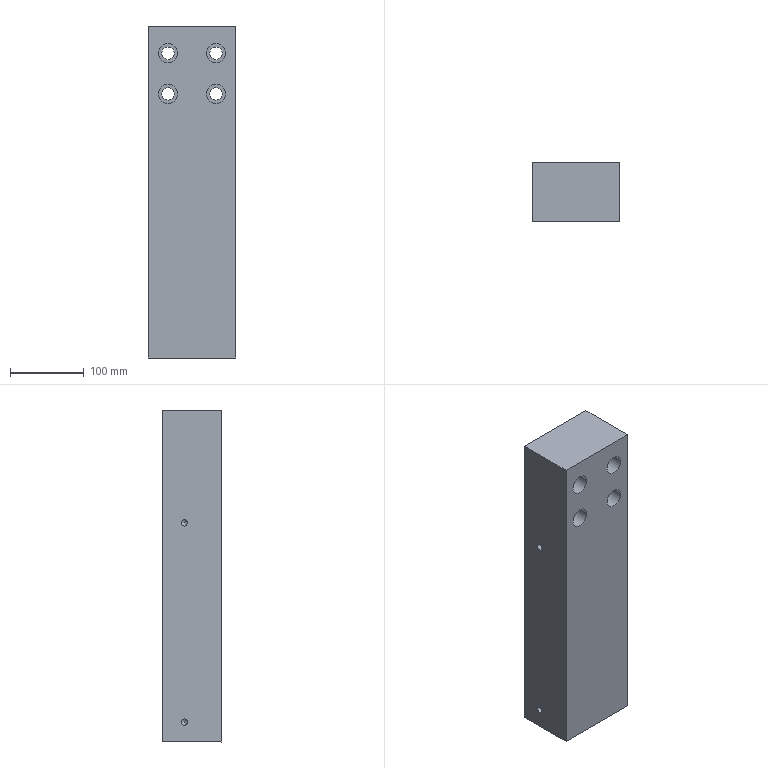Part | STEP file | lll_id1714_x_t | 1 solid | 42 faces | box 118 x 80 x 450 mm | volume 4104753 mm3 | cylinder 20 | cone 12 | plane 10 | commonest cylinder face diameters 8.5 x11 17 x4 26 x4 14 x1
STEP:
#1=CARTESIAN_POINT('',(2092.435,-628.,-262.832));
#2=VERTEX_POINT('',#1);
#3=CARTESIAN_POINT('',(2092.435,-635.,-262.832));
#4=DIRECTION('',(0.,0.000000092,-1.));
#5=DIRECTION('',(0.,1.,0.000000092));
#6=AXIS2_PLACEMENT_3D('',#3,#4,#5);
#7=CIRCLE('',#6,7.);
#8=EDGE_CURVE('',#2,#2,#7,.T.);
#9=ORIENTED_EDGE('',*,*,#8,.T.);
#10=EDGE_LOOP('',(#9));
#11=FACE_BOUND('',#10,.T.);
#12=CARTESIAN_POINT('',(2092.435,-635.,-258.626));
#13=VERTEX_POINT('',#12);
#14=VERTEX_LOOP('',#13);
#15=FACE_BOUND('',#14,.T.);
#16=CARTESIAN_POINT('',(2092.435,-635.,-262.213));
#17=DIRECTION('',(0.,0.000000092,-1.));
#18=DIRECTION('',(1.,0.,0.));
#19=AXIS2_PLACEMENT_3D('',#16,#17,#18);
#20=CONICAL_SURFACE('',#19,5.97,59.);
#21=ADVANCED_FACE('',(#11,#15),#20,.F.);
#22=CARTESIAN_POINT('',(2062.989,-625.5,9.5));
#23=VERTEX_POINT('',#22);
#24=VERTEX_LOOP('',#23);
#25=FACE_BOUND('',#24,.T.);
#26=CARTESIAN_POINT('',(2060.435,-625.5,13.75));
#27=VERTEX_POINT('',#26);
#28=CARTESIAN_POINT('',(2060.435,-625.5,9.5));
#29=DIRECTION('',(1.,0.,0.));
#30=DIRECTION('',(0.,-0.000000092,1.));
#31=AXIS2_PLACEMENT_3D('',#28,#29,#30);
#32=CIRCLE('',#31,4.25);
#33=EDGE_CURVE('',#27,#27,#32,.T.);
#34=ORIENTED_EDGE('',*,*,#33,.F.);
#35=EDGE_LOOP('',(#34));
#36=FACE_BOUND('',#35,.T.);
#37=CARTESIAN_POINT('',(2060.435,-625.5,9.5));
#38=DIRECTION('',(-1.,0.,0.));
#39=DIRECTION('',(0.,0.000000092,-1.));
#40=AXIS2_PLACEMENT_3D('',#37,#38,#39);
#41=CONICAL_SURFACE('',#40,4.25,59.);
#42=ADVANCED_FACE('',(#25,#36),#41,.F.);
#43=CARTESIAN_POINT('',(2062.989,-625.5,-260.5));
#44=VERTEX_POINT('',#43);
#45=VERTEX_LOOP('',#44);
#46=FACE_BOUND('',#45,.T.);
#47=CARTESIAN_POINT('',(2060.435,-625.5,-256.25));
#48=VERTEX_POINT('',#47);
#49=CARTESIAN_POINT('',(2060.435,-625.5,-260.5));
#50=DIRECTION('',(1.,0.,0.));
#51=DIRECTION('',(0.,-0.000000092,1.));
#52=AXIS2_PLACEMENT_3D('',#49,#50,#51);
#53=CIRCLE('',#52,4.25);
#54=EDGE_CURVE('',#48,#48,#53,.T.);
#55=ORIENTED_EDGE('',*,*,#54,.F.);
#56=EDGE_LOOP('',(#55));
#57=FACE_BOUND('',#56,.T.);
#58=CARTESIAN_POINT('',(2060.435,-625.5,-260.5));
#59=DIRECTION('',(-1.,0.,0.));
#60=DIRECTION('',(0.,0.000000092,-1.));
#61=AXIS2_PLACEMENT_3D('',#58,#59,#60);
#62=CONICAL_SURFACE('',#61,4.25,59.);
#63=ADVANCED_FACE('',(#46,#57),#62,.F.);
#64=CARTESIAN_POINT('',(2121.882,-625.5,9.5));
#65=VERTEX_POINT('',#64);
#66=VERTEX_LOOP('',#65);
#67=FACE_BOUND('',#66,.T.);
#68=CARTESIAN_POINT('',(2124.435,-625.5,13.75));
#69=VERTEX_POINT('',#68);
#70=CARTESIAN_POINT('',(2124.435,-625.5,9.5));
#71=DIRECTION('',(-1.,0.,0.));
#72=DIRECTION('',(0.,-0.000000092,1.));
#73=AXIS2_PLACEMENT_3D('',#70,#71,#72);
#74=CIRCLE('',#73,4.25);
#75=EDGE_CURVE('',#69,#69,#74,.T.);
#76=ORIENTED_EDGE('',*,*,#75,.F.);
#77=EDGE_LOOP('',(#76));
#78=FACE_BOUND('',#77,.T.);
#79=CARTESIAN_POINT('',(2124.435,-625.5,9.5));
#80=DIRECTION('',(1.,0.,0.));
#81=DIRECTION('',(0.,-0.000000092,1.));
#82=AXIS2_PLACEMENT_3D('',#79,#80,#81);
#83=CONICAL_SURFACE('',#82,4.25,59.);
#84=ADVANCED_FACE('',(#67,#78),#83,.F.);
#85=CARTESIAN_POINT('',(2121.882,-625.5,-260.5));
#86=VERTEX_POINT('',#85);
#87=VERTEX_LOOP('',#86);
#88=FACE_BOUND('',#87,.T.);
#89=CARTESIAN_POINT('',(2124.435,-625.5,-256.25));
#90=VERTEX_POINT('',#89);
#91=CARTESIAN_POINT('',(2124.435,-625.5,-260.5));
#92=DIRECTION('',(-1.,0.,0.));
#93=DIRECTION('',(0.,-0.000000092,1.));
#94=AXIS2_PLACEMENT_3D('',#91,#92,#93);
#95=CIRCLE('',#94,4.25);
#96=EDGE_CURVE('',#90,#90,#95,.T.);
#97=ORIENTED_EDGE('',*,*,#96,.F.);
#98=EDGE_LOOP('',(#97));
#99=FACE_BOUND('',#98,.T.);
#100=CARTESIAN_POINT('',(2124.435,-625.5,-260.5));
#101=DIRECTION('',(1.,0.,0.));
#102=DIRECTION('',(0.,-0.000000092,1.));
#103=AXIS2_PLACEMENT_3D('',#100,#101,#102);
#104=CONICAL_SURFACE('',#103,4.25,59.);
#105=ADVANCED_FACE('',(#88,#99),#104,.F.);
#106=CARTESIAN_POINT('',(2124.935,-636.5,83.5));
#107=VERTEX_POINT('',#106);
#108=CARTESIAN_POINT('',(2124.935,-636.5,70.5));
#109=DIRECTION('',(0.,-1.,-0.000000092));
#110=DIRECTION('',(0.,-0.000000092,1.));
#111=AXIS2_PLACEMENT_3D('',#108,#109,#110);
#112=CIRCLE('',#111,13.);
#113=EDGE_CURVE('',#107,#107,#112,.T.);
#114=ORIENTED_EDGE('',*,*,#113,.T.);
#115=EDGE_LOOP('',(#114));
#116=FACE_BOUND('',#115,.T.);
#117=CARTESIAN_POINT('',(2124.935,-636.5,79.));
#118=VERTEX_POINT('',#117);
#119=CARTESIAN_POINT('',(2124.935,-636.5,70.5));
#120=DIRECTION('',(0.,1.,0.000000092));
#121=DIRECTION('',(0.,-0.000000092,1.));
#122=AXIS2_PLACEMENT_3D('',#119,#120,#121);
#123=CIRCLE('',#122,8.5);
#124=EDGE_CURVE('',#118,#118,#123,.T.);
#125=ORIENTED_EDGE('',*,*,#124,.T.);
#126=EDGE_LOOP('',(#125));
#127=FACE_BOUND('',#126,.T.);
#128=CARTESIAN_POINT('',(2124.935,-636.5,70.5));
#129=DIRECTION('',(0.,1.,0.000000092));
#130=DIRECTION('',(0.,0.000000092,-1.));
#131=AXIS2_PLACEMENT_3D('',#128,#129,#130);
#132=PLANE('',#131);
#133=ADVANCED_FACE('',(#116,#127),#132,.F.);
#134=CARTESIAN_POINT('',(2059.935,-636.5,112.5));
#135=VERTEX_POINT('',#134);
#136=CARTESIAN_POINT('',(2059.935,-636.5,125.5));
#137=DIRECTION('',(0.,1.,0.000000092));
#138=DIRECTION('',(0.,0.000000092,-1.));
#139=AXIS2_PLACEMENT_3D('',#136,#137,#138);
#140=CIRCLE('',#139,13.);
#141=EDGE_CURVE('',#135,#135,#140,.T.);
#142=ORIENTED_EDGE('',*,*,#141,.F.);
#143=EDGE_LOOP('',(#142));
#144=FACE_BOUND('',#143,.T.);
#145=CARTESIAN_POINT('',(2059.935,-636.5,117.));
#146=VERTEX_POINT('',#145);
#147=CARTESIAN_POINT('',(2059.935,-636.5,125.5));
#148=DIRECTION('',(0.,-1.,-0.000000092));
#149=DIRECTION('',(0.,0.000000092,-1.));
#150=AXIS2_PLACEMENT_3D('',#147,#148,#149);
#151=CIRCLE('',#150,8.5);
#152=EDGE_CURVE('',#146,#146,#151,.T.);
#153=ORIENTED_EDGE('',*,*,#152,.F.);
#154=EDGE_LOOP('',(#153));
#155=FACE_BOUND('',#154,.T.);
#156=CARTESIAN_POINT('',(2059.935,-636.5,110.5));
#157=DIRECTION('',(0.,-1.,-0.000000092));
#158=DIRECTION('',(0.,-0.000000092,1.));
#159=AXIS2_PLACEMENT_3D('',#156,#157,#158);
#160=PLANE('',#159);
#161=ADVANCED_FACE('',(#144,#155),#160,.T.);
#162=CARTESIAN_POINT('',(2059.935,-636.5,57.5));
#163=VERTEX_POINT('',#162);
#164=CARTESIAN_POINT('',(2059.935,-636.5,70.5));
#165=DIRECTION('',(0.,1.,0.000000092));
#166=DIRECTION('',(0.,0.000000092,-1.));
#167=AXIS2_PLACEMENT_3D('',#164,#165,#166);
#168=CIRCLE('',#167,13.);
#169=EDGE_CURVE('',#163,#163,#168,.T.);
#170=ORIENTED_EDGE('',*,*,#169,.F.);
#171=EDGE_LOOP('',(#170));
#172=FACE_BOUND('',#171,.T.);
#173=CARTESIAN_POINT('',(2059.935,-636.5,62.));
#174=VERTEX_POINT('',#173);
#175=CARTESIAN_POINT('',(2059.935,-636.5,70.5));
#176=DIRECTION('',(0.,-1.,-0.000000092));
#177=DIRECTION('',(0.,0.000000092,-1.));
#178=AXIS2_PLACEMENT_3D('',#175,#176,#177);
#179=CIRCLE('',#178,8.5);
#180=EDGE_CURVE('',#174,#174,#179,.T.);
#181=ORIENTED_EDGE('',*,*,#180,.F.);
#182=EDGE_LOOP('',(#181));
#183=FACE_BOUND('',#182,.T.);
#184=CARTESIAN_POINT('',(2059.935,-636.5,70.5));
#185=DIRECTION('',(0.,-1.,-0.000000092));
#186=DIRECTION('',(0.,-0.000000092,1.));
#187=AXIS2_PLACEMENT_3D('',#184,#185,#186);
#188=PLANE('',#187);
#189=ADVANCED_FACE('',(#172,#183),#188,.T.);
#190=CARTESIAN_POINT('',(2124.935,-636.5,138.5));
#191=VERTEX_POINT('',#190);
#192=CARTESIAN_POINT('',(2124.935,-636.5,125.5));
#193=DIRECTION('',(0.,-1.,-0.000000092));
#194=DIRECTION('',(0.,-0.000000092,1.));
#195=AXIS2_PLACEMENT_3D('',#192,#193,#194);
#196=CIRCLE('',#195,13.);
#197=EDGE_CURVE('',#191,#191,#196,.T.);
#198=ORIENTED_EDGE('',*,*,#197,.T.);
#199=EDGE_LOOP('',(#198));
#200=FACE_BOUND('',#199,.T.);
#201=CARTESIAN_POINT('',(2124.935,-636.5,134.));
#202=VERTEX_POINT('',#201);
#203=CARTESIAN_POINT('',(2124.935,-636.5,125.5));
#204=DIRECTION('',(0.,1.,0.000000092));
#205=DIRECTION('',(0.,-0.000000092,1.));
#206=AXIS2_PLACEMENT_3D('',#203,#204,#205);
#207=CIRCLE('',#206,8.5);
#208=EDGE_CURVE('',#202,#202,#207,.T.);
#209=ORIENTED_EDGE('',*,*,#208,.T.);
#210=EDGE_LOOP('',(#209));
#211=FACE_BOUND('',#210,.T.);
#212=CARTESIAN_POINT('',(2124.935,-636.5,110.5));
#213=DIRECTION('',(0.,1.,0.000000092));
#214=DIRECTION('',(0.,0.000000092,-1.));
#215=AXIS2_PLACEMENT_3D('',#212,#213,#214);
#216=PLANE('',#215);
#217=ADVANCED_FACE('',(#200,#211),#216,.F.);
#218=ORIENTED_EDGE('',*,*,#8,.F.);
#219=EDGE_LOOP('',(#218));
#220=FACE_BOUND('',#219,.T.);
#221=CARTESIAN_POINT('',(2092.435,-642.,-287.5));
#222=VERTEX_POINT('',#221);
#223=CARTESIAN_POINT('',(2092.435,-635.,-287.5));
#224=DIRECTION('',(0.,0.000000092,-1.));
#225=DIRECTION('',(0.,-1.,-0.000000092));
#226=AXIS2_PLACEMENT_3D('',#223,#224,#225);
#227=CIRCLE('',#226,7.);
#228=EDGE_CURVE('',#222,#222,#227,.T.);
#229=ORIENTED_EDGE('',*,*,#228,.T.);
#230=EDGE_LOOP('',(#229));
#231=FACE_BOUND('',#230,.T.);
#232=CARTESIAN_POINT('',(2092.435,-635.,-255.5));
#233=DIRECTION('',(0.,-0.000000092,1.));
#234=DIRECTION('',(-1.,0.,0.));
#235=AXIS2_PLACEMENT_3D('',#232,#233,#234);
#236=CYLINDRICAL_SURFACE('',#235,7.);
#237=ADVANCED_FACE('',(#220,#231),#236,.F.);
#238=ORIENTED_EDGE('',*,*,#33,.T.);
#239=EDGE_LOOP('',(#238));
#240=FACE_BOUND('',#239,.T.);
#241=CARTESIAN_POINT('',(2033.435,-625.5,5.25));
#242=VERTEX_POINT('',#241);
#243=CARTESIAN_POINT('',(2033.435,-625.5,9.5));
#244=DIRECTION('',(1.,0.,0.));
#245=DIRECTION('',(0.,0.,-1.));
#246=AXIS2_PLACEMENT_3D('',#243,#244,#245);
#247=CIRCLE('',#246,4.25);
#248=EDGE_CURVE('',#242,#242,#247,.T.);
#249=ORIENTED_EDGE('',*,*,#248,.F.);
#250=EDGE_LOOP('',(#249));
#251=FACE_BOUND('',#250,.T.);
#252=CARTESIAN_POINT('',(2064.935,-625.5,9.5));
#253=DIRECTION('',(1.,0.,0.));
#254=DIRECTION('',(0.,-0.000000092,1.));
#255=AXIS2_PLACEMENT_3D('',#252,#253,#254);
#256=CYLINDRICAL_SURFACE('',#255,4.25);
#257=ADVANCED_FACE('',(#240,#251),#256,.F.);
#258=ORIENTED_EDGE('',*,*,#54,.T.);
#259=EDGE_LOOP('',(#258));
#260=FACE_BOUND('',#259,.T.);
#261=CARTESIAN_POINT('',(2033.435,-625.5,-264.75));
#262=VERTEX_POINT('',#261);
#263=CARTESIAN_POINT('',(2033.435,-625.5,-260.5));
#264=DIRECTION('',(1.,0.,0.));
#265=DIRECTION('',(0.,0.,-1.));
#266=AXIS2_PLACEMENT_3D('',#263,#264,#265);
#267=CIRCLE('',#266,4.25);
#268=EDGE_CURVE('',#262,#262,#267,.T.);
#269=ORIENTED_EDGE('',*,*,#268,.F.);
#270=EDGE_LOOP('',(#269));
#271=FACE_BOUND('',#270,.T.);
#272=CARTESIAN_POINT('',(2064.935,-625.5,-260.5));
#273=DIRECTION('',(1.,0.,0.));
#274=DIRECTION('',(0.,-0.000000092,1.));
#275=AXIS2_PLACEMENT_3D('',#272,#273,#274);
#276=CYLINDRICAL_SURFACE('',#275,4.25);
#277=ADVANCED_FACE('',(#260,#271),#276,.F.);
#278=ORIENTED_EDGE('',*,*,#75,.T.);
#279=EDGE_LOOP('',(#278));
#280=FACE_BOUND('',#279,.T.);
#281=CARTESIAN_POINT('',(2151.435,-625.5,13.75));
#282=VERTEX_POINT('',#281);
#283=CARTESIAN_POINT('',(2151.435,-625.5,9.5));
#284=DIRECTION('',(-1.,0.,0.));
#285=DIRECTION('',(0.,0.,1.));
#286=AXIS2_PLACEMENT_3D('',#283,#284,#285);
#287=CIRCLE('',#286,4.25);
#288=EDGE_CURVE('',#282,#282,#287,.T.);
#289=ORIENTED_EDGE('',*,*,#288,.F.);
#290=EDGE_LOOP('',(#289));
#291=FACE_BOUND('',#290,.T.);
#292=CARTESIAN_POINT('',(2119.935,-625.5,9.5));
#293=DIRECTION('',(-1.,0.,0.));
#294=DIRECTION('',(0.,0.000000092,-1.));
#295=AXIS2_PLACEMENT_3D('',#292,#293,#294);
#296=CYLINDRICAL_SURFACE('',#295,4.25);
#297=ADVANCED_FACE('',(#280,#291),#296,.F.);
#298=ORIENTED_EDGE('',*,*,#96,.T.);
#299=EDGE_LOOP('',(#298));
#300=FACE_BOUND('',#299,.T.);
#301=CARTESIAN_POINT('',(2151.435,-625.5,-256.25));
#302=VERTEX_POINT('',#301);
#303=CARTESIAN_POINT('',(2151.435,-625.5,-260.5));
#304=DIRECTION('',(-1.,0.,0.));
#305=DIRECTION('',(0.,0.,1.));
#306=AXIS2_PLACEMENT_3D('',#303,#304,#305);
#307=CIRCLE('',#306,4.25);
#308=EDGE_CURVE('',#302,#302,#307,.T.);
#309=ORIENTED_EDGE('',*,*,#308,.F.);
#310=EDGE_LOOP('',(#309));
#311=FACE_BOUND('',#310,.T.);
#312=CARTESIAN_POINT('',(2119.935,-625.5,-260.5));
#313=DIRECTION('',(-1.,0.,0.));
#314=DIRECTION('',(0.,0.000000092,-1.));
#315=AXIS2_PLACEMENT_3D('',#312,#313,#314);
#316=CYLINDRICAL_SURFACE('',#315,4.25);
#317=ADVANCED_FACE('',(#300,#311),#316,.F.);
#318=ORIENTED_EDGE('',*,*,#124,.F.);
#319=EDGE_LOOP('',(#318));
#320=FACE_BOUND('',#319,.T.);
#321=CARTESIAN_POINT('',(2124.935,-596.,62.));
#322=VERTEX_POINT('',#321);
#323=CARTESIAN_POINT('',(2124.935,-596.,70.5));
#324=DIRECTION('',(0.,1.,0.000000092));
#325=DIRECTION('',(0.,0.000000092,-1.));
#326=AXIS2_PLACEMENT_3D('',#323,#324,#325);
#327=CIRCLE('',#326,8.5);
#328=EDGE_CURVE('',#322,#322,#327,.T.);
#329=ORIENTED_EDGE('',*,*,#328,.T.);
#330=EDGE_LOOP('',(#329));
#331=FACE_BOUND('',#330,.T.);
#332=CARTESIAN_POINT('',(2124.935,-649.5,70.5));
#333=DIRECTION('',(0.,1.,0.000000092));
#334=DIRECTION('',(0.,0.000000092,-1.));
#335=AXIS2_PLACEMENT_3D('',#332,#333,#334);
#336=CYLINDRICAL_SURFACE('',#335,8.5);
#337=ADVANCED_FACE('',(#320,#331),#336,.F.);
#338=ORIENTED_EDGE('',*,*,#152,.T.);
#339=EDGE_LOOP('',(#338));
#340=FACE_BOUND('',#339,.T.);
#341=CARTESIAN_POINT('',(2059.935,-596.,117.));
#342=VERTEX_POINT('',#341);
#343=CARTESIAN_POINT('',(2059.935,-596.,125.5));
#344=DIRECTION('',(0.,1.,0.000000092));
#345=DIRECTION('',(0.,0.000000092,-1.));
#346=AXIS2_PLACEMENT_3D('',#343,#344,#345);
#347=CIRCLE('',#346,8.5);
#348=EDGE_CURVE('',#342,#342,#347,.T.);
#349=ORIENTED_EDGE('',*,*,#348,.T.);
#350=EDGE_LOOP('',(#349));
#351=FACE_BOUND('',#350,.T.);
#352=CARTESIAN_POINT('',(2059.935,-649.5,125.5));
#353=DIRECTION('',(0.,1.,0.000000092));
#354=DIRECTION('',(0.,0.000000092,-1.));
#355=AXIS2_PLACEMENT_3D('',#352,#353,#354);
#356=CYLINDRICAL_SURFACE('',#355,8.5);
#357=ADVANCED_FACE('',(#340,#351),#356,.F.);
#358=ORIENTED_EDGE('',*,*,#180,.T.);
#359=EDGE_LOOP('',(#358));
#360=FACE_BOUND('',#359,.T.);
#361=CARTESIAN_POINT('',(2059.935,-596.,62.));
#362=VERTEX_POINT('',#361);
#363=CARTESIAN_POINT('',(2059.935,-596.,70.5));
#364=DIRECTION('',(0.,1.,0.000000092));
#365=DIRECTION('',(0.,0.000000092,-1.));
#366=AXIS2_PLACEMENT_3D('',#363,#364,#365);
#367=CIRCLE('',#366,8.5);
#368=EDGE_CURVE('',#362,#362,#367,.T.);
#369=ORIENTED_EDGE('',*,*,#368,.T.);
#370=EDGE_LOOP('',(#369));
#371=FACE_BOUND('',#370,.T.);
#372=CARTESIAN_POINT('',(2059.935,-649.5,70.5));
#373=DIRECTION('',(0.,1.,0.000000092));
#374=DIRECTION('',(0.,0.000000092,-1.));
#375=AXIS2_PLACEMENT_3D('',#372,#373,#374);
#376=CYLINDRICAL_SURFACE('',#375,8.5);
#377=ADVANCED_FACE('',(#360,#371),#376,.F.);
#378=ORIENTED_EDGE('',*,*,#208,.F.);
#379=EDGE_LOOP('',(#378));
#380=FACE_BOUND('',#379,.T.);
#381=CARTESIAN_POINT('',(2124.935,-596.,117.));
#382=VERTEX_POINT('',#381);
#383=CARTESIAN_POINT('',(2124.935,-596.,125.5));
#384=DIRECTION('',(0.,1.,0.000000092));
#385=DIRECTION('',(0.,0.000000092,-1.));
#386=AXIS2_PLACEMENT_3D('',#383,#384,#385);
#387=CIRCLE('',#386,8.5);
#388=EDGE_CURVE('',#382,#382,#387,.T.);
#389=ORIENTED_EDGE('',*,*,#388,.T.);
#390=EDGE_LOOP('',(#389));
#391=FACE_BOUND('',#390,.T.);
#392=CARTESIAN_POINT('',(2124.935,-649.5,125.5));
#393=DIRECTION('',(0.,1.,0.000000092));
#394=DIRECTION('',(0.,0.000000092,-1.));
#395=AXIS2_PLACEMENT_3D('',#392,#393,#394);
#396=CYLINDRICAL_SURFACE('',#395,8.5);
#397=ADVANCED_FACE('',(#380,#391),#396,.F.);
#398=ORIENTED_EDGE('',*,*,#228,.F.);
#399=EDGE_LOOP('',(#398));
#400=FACE_BOUND('',#399,.T.);
#401=CARTESIAN_POINT('',(2151.435,-676.,-287.5));
#402=VERTEX_POINT('',#401);
#403=CARTESIAN_POINT('',(2151.435,-596.,-287.5));
#404=VERTEX_POINT('',#403);
#405=CARTESIAN_POINT('',(2151.435,-604.571,-287.5));
#406=DIRECTION('',(0.,1.,0.000000092));
#407=VECTOR('',#406,1.);
#408=LINE('',#405,#407);
#409=EDGE_CURVE('',#402,#404,#408,.T.);
#410=ORIENTED_EDGE('',*,*,#409,.F.);
#411=CARTESIAN_POINT('',(2033.435,-676.,-287.5));
#412=VERTEX_POINT('',#411);
#413=CARTESIAN_POINT('',(2029.935,-676.,-287.5));
#414=DIRECTION('',(-1.,0.,0.));
#415=VECTOR('',#414,1.);
#416=LINE('',#413,#415);
#417=EDGE_CURVE('',#402,#412,#416,.T.);
#418=ORIENTED_EDGE('',*,*,#417,.T.);
#419=CARTESIAN_POINT('',(2033.435,-596.,-287.5));
#420=VERTEX_POINT('',#419);
#421=CARTESIAN_POINT('',(2033.435,-604.571,-287.5));
#422=DIRECTION('',(0.,-1.,-0.000000092));
#423=VECTOR('',#422,1.);
#424=LINE('',#421,#423);
#425=EDGE_CURVE('',#420,#412,#424,.T.);
#426=ORIENTED_EDGE('',*,*,#425,.F.);
#427=CARTESIAN_POINT('',(2149.935,-596.,-287.5));
#428=DIRECTION('',(1.,0.,0.));
#429=VECTOR('',#428,1.);
#430=LINE('',#427,#429);
#431=EDGE_CURVE('',#420,#404,#430,.T.);
#432=ORIENTED_EDGE('',*,*,#431,.T.);
#433=EDGE_LOOP('',(#410,#418,#426,#432));
#434=FACE_BOUND('',#433,.T.);
#435=CARTESIAN_POINT('',(2149.935,-604.571,-287.5));
#436=DIRECTION('',(0.,-0.000000092,1.));
#437=DIRECTION('',(-1.,0.,0.));
#438=AXIS2_PLACEMENT_3D('',#435,#436,#437);
#439=PLANE('',#438);
#440=ADVANCED_FACE('',(#400,#434),#439,.F.);
#441=ORIENTED_EDGE('',*,*,#268,.T.);
#442=EDGE_LOOP('',(#441));
#443=FACE_BOUND('',#442,.T.);
#444=ORIENTED_EDGE('',*,*,#248,.T.);
#445=EDGE_LOOP('',(#444));
#446=FACE_BOUND('',#445,.T.);
#447=CARTESIAN_POINT('',(2033.435,-596.,162.5));
#448=VERTEX_POINT('',#447);
#449=CARTESIAN_POINT('',(2033.435,-596.,-85.484));
#450=DIRECTION('',(0.,0.000000092,-1.));
#451=VECTOR('',#450,1.);
#452=LINE('',#449,#451);
#453=EDGE_CURVE('',#448,#420,#452,.T.);
#454=ORIENTED_EDGE('',*,*,#453,.T.);
#455=ORIENTED_EDGE('',*,*,#425,.T.);
#456=CARTESIAN_POINT('',(2033.435,-676.,162.5));
#457=VERTEX_POINT('',#456);
#458=CARTESIAN_POINT('',(2033.435,-676.,180.5));
#459=DIRECTION('',(0.,0.000000092,-1.));
#460=VECTOR('',#459,1.);
#461=LINE('',#458,#460);
#462=EDGE_CURVE('',#457,#412,#461,.T.);
#463=ORIENTED_EDGE('',*,*,#462,.F.);
#464=CARTESIAN_POINT('',(2033.435,-549.5,162.5));
#465=DIRECTION('',(0.,-1.,-0.000000092));
#466=VECTOR('',#465,1.);
#467=LINE('',#464,#466);
#468=EDGE_CURVE('',#448,#457,#467,.T.);
#469=ORIENTED_EDGE('',*,*,#468,.F.);
#470=EDGE_LOOP('',(#454,#455,#463,#469));
#471=FACE_BOUND('',#470,.T.);
#472=CARTESIAN_POINT('',(2033.435,-549.5,-85.484));
#473=DIRECTION('',(-1.,0.,0.));
#474=DIRECTION('',(0.,0.000000092,-1.));
#475=AXIS2_PLACEMENT_3D('',#472,#473,#474);
#476=PLANE('',#475);
#477=ADVANCED_FACE('',(#443,#446,#471),#476,.T.);
#478=ORIENTED_EDGE('',*,*,#468,.T.);
#479=CARTESIAN_POINT('',(2151.435,-676.,162.5));
#480=VERTEX_POINT('',#479);
#481=CARTESIAN_POINT('',(2029.935,-676.,162.5));
#482=DIRECTION('',(-1.,0.,0.));
#483=VECTOR('',#482,1.);
#484=LINE('',#481,#483);
#485=EDGE_CURVE('',#480,#457,#484,.T.);
#486=ORIENTED_EDGE('',*,*,#485,.F.);
#487=CARTESIAN_POINT('',(2151.435,-596.,162.5));
#488=VERTEX_POINT('',#487);
#489=CARTESIAN_POINT('',(2151.435,-574.,162.5));
#490=DIRECTION('',(0.,-1.,-0.000000092));
#491=VECTOR('',#490,1.);
#492=LINE('',#489,#491);
#493=EDGE_CURVE('',#488,#480,#492,.T.);
#494=ORIENTED_EDGE('',*,*,#493,.F.);
#495=CARTESIAN_POINT('',(2157.935,-596.,162.5));
#496=DIRECTION('',(1.,0.,0.));
#497=VECTOR('',#496,1.);
#498=LINE('',#495,#497);
#499=EDGE_CURVE('',#448,#488,#498,.T.);
#500=ORIENTED_EDGE('',*,*,#499,.F.);
#501=EDGE_LOOP('',(#478,#486,#494,#500));
#502=FACE_OUTER_BOUND('',#501,.T.);
#503=CARTESIAN_POINT('',(2034.935,-574.,162.5));
#504=DIRECTION('',(0.,-0.000000092,1.));
#505=DIRECTION('',(1.,0.,0.));
#506=AXIS2_PLACEMENT_3D('',#503,#504,#505);
#507=PLANE('',#506);
#508=ADVANCED_FACE('',(#502),#507,.T.);
#509=CARTESIAN_POINT('',(2151.435,-625.5,-121.25));
#510=VERTEX_POINT('',#509);
#511=CARTESIAN_POINT('',(2151.435,-625.5,-125.5));
#512=DIRECTION('',(-1.,0.,0.));
#513=DIRECTION('',(0.,0.,1.));
#514=AXIS2_PLACEMENT_3D('',#511,#512,#513);
#515=CIRCLE('',#514,4.25);
#516=EDGE_CURVE('',#510,#510,#515,.T.);
#517=ORIENTED_EDGE('',*,*,#516,.T.);
#518=EDGE_LOOP('',(#517));
#519=FACE_BOUND('',#518,.T.);
#520=ORIENTED_EDGE('',*,*,#308,.T.);
#521=EDGE_LOOP('',(#520));
#522=FACE_BOUND('',#521,.T.);
#523=ORIENTED_EDGE('',*,*,#288,.T.);
#524=EDGE_LOOP('',(#523));
#525=FACE_BOUND('',#524,.T.);
#526=CARTESIAN_POINT('',(2151.435,-676.,180.5));
#527=DIRECTION('',(0.,-0.000000092,1.));
#528=VECTOR('',#527,1.);
#529=LINE('',#526,#528);
#530=EDGE_CURVE('',#402,#480,#529,.T.);
#531=ORIENTED_EDGE('',*,*,#530,.F.);
#532=ORIENTED_EDGE('',*,*,#409,.T.);
#533=CARTESIAN_POINT('',(2151.435,-596.,24.5));
#534=DIRECTION('',(0.,0.000000092,-1.));
#535=VECTOR('',#534,1.);
#536=LINE('',#533,#535);
#537=EDGE_CURVE('',#488,#404,#536,.T.);
#538=ORIENTED_EDGE('',*,*,#537,.F.);
#539=ORIENTED_EDGE('',*,*,#493,.T.);
#540=EDGE_LOOP('',(#531,#532,#538,#539));
#541=FACE_BOUND('',#540,.T.);
#542=CARTESIAN_POINT('',(2151.435,-549.5,49.509));
#543=DIRECTION('',(1.,0.,0.));
#544=DIRECTION('',(0.,-0.000000092,1.));
#545=AXIS2_PLACEMENT_3D('',#542,#543,#544);
#546=PLANE('',#545);
#547=ADVANCED_FACE('',(#519,#522,#525,#541),#546,.T.);
#548=CARTESIAN_POINT('',(2067.435,-596.,-103.75));
#549=VERTEX_POINT('',#548);
#550=CARTESIAN_POINT('',(2067.435,-596.,-108.));
#551=DIRECTION('',(0.,1.,0.000000092));
#552=DIRECTION('',(0.,-0.000000092,1.));
#553=AXIS2_PLACEMENT_3D('',#550,#551,#552);
#554=CIRCLE('',#553,4.25);
#555=EDGE_CURVE('',#549,#549,#554,.T.);
#556=ORIENTED_EDGE('',*,*,#555,.F.);
#557=EDGE_LOOP('',(#556));
#558=FACE_BOUND('',#557,.T.);
#559=CARTESIAN_POINT('',(2117.435,-596.,-103.75));
#560=VERTEX_POINT('',#559);
#561=CARTESIAN_POINT('',(2117.435,-596.,-108.));
#562=DIRECTION('',(0.,1.,0.000000092));
#563=DIRECTION('',(0.,-0.000000092,1.));
#564=AXIS2_PLACEMENT_3D('',#561,#562,#563);
#565=CIRCLE('',#564,4.25);
#566=EDGE_CURVE('',#560,#560,#565,.T.);
#567=ORIENTED_EDGE('',*,*,#566,.F.);
#568=EDGE_LOOP('',(#567));
#569=FACE_BOUND('',#568,.T.);
#570=CARTESIAN_POINT('',(2067.435,-596.,23.75));
#571=VERTEX_POINT('',#570);
#572=CARTESIAN_POINT('',(2067.435,-596.,19.5));
#573=DIRECTION('',(0.,1.,0.000000092));
#574=DIRECTION('',(0.,-0.000000092,1.));
#575=AXIS2_PLACEMENT_3D('',#572,#573,#574);
#576=CIRCLE('',#575,4.25);
#577=EDGE_CURVE('',#571,#571,#576,.T.);
#578=ORIENTED_EDGE('',*,*,#577,.F.);
#579=EDGE_LOOP('',(#578));
#580=FACE_BOUND('',#579,.T.);
#581=CARTESIAN_POINT('',(2117.435,-596.,23.75));
#582=VERTEX_POINT('',#581);
#583=CARTESIAN_POINT('',(2117.435,-596.,19.5));
#584=DIRECTION('',(0.,1.,0.000000092));
#585=DIRECTION('',(0.,-0.000000092,1.));
#586=AXIS2_PLACEMENT_3D('',#583,#584,#585);
#587=CIRCLE('',#586,4.25);
#588=EDGE_CURVE('',#582,#582,#587,.T.);
#589=ORIENTED_EDGE('',*,*,#588,.F.);
#590=EDGE_LOOP('',(#589));
#591=FACE_BOUND('',#590,.T.);
#592=CARTESIAN_POINT('',(2117.435,-596.,-241.25));
#593=VERTEX_POINT('',#592);
#594=CARTESIAN_POINT('',(2117.435,-596.,-245.5));
#595=DIRECTION('',(0.,1.,0.000000092));
#596=DIRECTION('',(0.,-0.000000092,1.));
#597=AXIS2_PLACEMENT_3D('',#594,#595,#596);
#598=CIRCLE('',#597,4.25);
#599=EDGE_CURVE('',#593,#593,#598,.T.);
#600=ORIENTED_EDGE('',*,*,#599,.F.);
#601=EDGE_LOOP('',(#600));
#602=FACE_BOUND('',#601,.T.);
#603=CARTESIAN_POINT('',(2067.435,-596.,-241.25));
#604=VERTEX_POINT('',#603);
#605=CARTESIAN_POINT('',(2067.435,-596.,-245.5));
#606=DIRECTION('',(0.,1.,0.000000092));
#607=DIRECTION('',(0.,-0.000000092,1.));
#608=AXIS2_PLACEMENT_3D('',#605,#606,#607);
#609=CIRCLE('',#608,4.25);
#610=EDGE_CURVE('',#604,#604,#609,.T.);
#611=ORIENTED_EDGE('',*,*,#610,.F.);
#612=EDGE_LOOP('',(#611));
#613=FACE_BOUND('',#612,.T.);
#614=ORIENTED_EDGE('',*,*,#537,.T.);
#615=ORIENTED_EDGE('',*,*,#431,.F.);
#616=ORIENTED_EDGE('',*,*,#453,.F.);
#617=ORIENTED_EDGE('',*,*,#499,.T.);
#618=EDGE_LOOP('',(#614,#615,#616,#617));
#619=FACE_BOUND('',#618,.T.);
#620=ORIENTED_EDGE('',*,*,#388,.F.);
#621=EDGE_LOOP('',(#620));
#622=FACE_BOUND('',#621,.T.);
#623=ORIENTED_EDGE('',*,*,#368,.F.);
#624=EDGE_LOOP('',(#623));
#625=FACE_BOUND('',#624,.T.);
#626=ORIENTED_EDGE('',*,*,#348,.F.);
#627=EDGE_LOOP('',(#626));
#628=FACE_BOUND('',#627,.T.);
#629=ORIENTED_EDGE('',*,*,#328,.F.);
#630=EDGE_LOOP('',(#629));
#631=FACE_BOUND('',#630,.T.);
#632=CARTESIAN_POINT('',(2157.935,-596.,24.5));
#633=DIRECTION('',(0.,-1.,-0.000000092));
#634=DIRECTION('',(0.,0.000000092,-1.));
#635=AXIS2_PLACEMENT_3D('',#632,#633,#634);
#636=PLANE('',#635);
#637=ADVANCED_FACE('',(#558,#569,#580,#591,#602,#613,#619,#622,#625,#628,#631),#636,.F.);
#638=CARTESIAN_POINT('',(2059.935,-676.,57.5));
#639=VERTEX_POINT('',#638);
#640=CARTESIAN_POINT('',(2059.935,-676.,70.5));
#641=DIRECTION('',(0.,-1.,-0.000000092));
#642=DIRECTION('',(0.,0.000000092,-1.));
#643=AXIS2_PLACEMENT_3D('',#640,#641,#642);
#644=CIRCLE('',#643,13.);
#645=EDGE_CURVE('',#639,#639,#644,.T.);
#646=ORIENTED_EDGE('',*,*,#645,.T.);
#647=EDGE_LOOP('',(#646));
#648=FACE_BOUND('',#647,.T.);
#649=ORIENTED_EDGE('',*,*,#169,.T.);
#650=EDGE_LOOP('',(#649));
#651=FACE_BOUND('',#650,.T.);
#652=CARTESIAN_POINT('',(2059.935,-649.5,70.5));
#653=DIRECTION('',(0.,1.,0.000000092));
#654=DIRECTION('',(0.,0.000000092,-1.));
#655=AXIS2_PLACEMENT_3D('',#652,#653,#654);
#656=CYLINDRICAL_SURFACE('',#655,13.);
#657=ADVANCED_FACE('',(#648,#651),#656,.F.);
#658=CARTESIAN_POINT('',(2124.935,-676.,57.5));
#659=VERTEX_POINT('',#658);
#660=CARTESIAN_POINT('',(2124.935,-676.,70.5));
#661=DIRECTION('',(0.,1.,0.000000092));
#662=DIRECTION('',(0.,0.000000092,-1.));
#663=AXIS2_PLACEMENT_3D('',#660,#661,#662);
#664=CIRCLE('',#663,13.);
#665=EDGE_CURVE('',#659,#659,#664,.T.);
#666=ORIENTED_EDGE('',*,*,#665,.F.);
#667=EDGE_LOOP('',(#666));
#668=FACE_BOUND('',#667,.T.);
#669=ORIENTED_EDGE('',*,*,#113,.F.);
#670=EDGE_LOOP('',(#669));
#671=FACE_BOUND('',#670,.T.);
#672=CARTESIAN_POINT('',(2124.935,-649.5,70.5));
#673=DIRECTION('',(0.,1.,0.000000092));
#674=DIRECTION('',(0.,0.000000092,-1.));
#675=AXIS2_PLACEMENT_3D('',#672,#673,#674);
#676=CYLINDRICAL_SURFACE('',#675,13.);
#677=ADVANCED_FACE('',(#668,#671),#676,.F.);
#678=CARTESIAN_POINT('',(2059.935,-676.,112.5));
#679=VERTEX_POINT('',#678);
#680=CARTESIAN_POINT('',(2059.935,-676.,125.5));
#681=DIRECTION('',(0.,1.,0.000000092));
#682=DIRECTION('',(0.,0.000000092,-1.));
#683=AXIS2_PLACEMENT_3D('',#680,#681,#682);
#684=CIRCLE('',#683,13.);
#685=EDGE_CURVE('',#679,#679,#684,.T.);
#686=ORIENTED_EDGE('',*,*,#685,.F.);
#687=EDGE_LOOP('',(#686));
#688=FACE_BOUND('',#687,.T.);
#689=ORIENTED_EDGE('',*,*,#141,.T.);
#690=EDGE_LOOP('',(#689));
#691=FACE_BOUND('',#690,.T.);
#692=CARTESIAN_POINT('',(2059.935,-649.5,125.5));
#693=DIRECTION('',(0.,1.,0.000000092));
#694=DIRECTION('',(0.,0.000000092,-1.));
#695=AXIS2_PLACEMENT_3D('',#692,#693,#694);
#696=CYLINDRICAL_SURFACE('',#695,13.);
#697=ADVANCED_FACE('',(#688,#691),#696,.F.);
#698=CARTESIAN_POINT('',(2124.935,-676.,112.5));
#699=VERTEX_POINT('',#698);
#700=CARTESIAN_POINT('',(2124.935,-676.,125.5));
#701=DIRECTION('',(0.,-1.,-0.000000092));
#702=DIRECTION('',(0.,0.000000092,-1.));
#703=AXIS2_PLACEMENT_3D('',#700,#701,#702);
#704=CIRCLE('',#703,13.);
#705=EDGE_CURVE('',#699,#699,#704,.T.);
#706=ORIENTED_EDGE('',*,*,#705,.T.);
#707=EDGE_LOOP('',(#706));
#708=FACE_BOUND('',#707,.T.);
#709=ORIENTED_EDGE('',*,*,#197,.F.);
#710=EDGE_LOOP('',(#709));
#711=FACE_BOUND('',#710,.T.);
#712=CARTESIAN_POINT('',(2124.935,-649.5,125.5));
#713=DIRECTION('',(0.,1.,0.000000092));
#714=DIRECTION('',(0.,0.000000092,-1.));
#715=AXIS2_PLACEMENT_3D('',#712,#713,#714);
#716=CYLINDRICAL_SURFACE('',#715,13.);
#717=ADVANCED_FACE('',(#708,#711),#716,.F.);
#718=ORIENTED_EDGE('',*,*,#705,.F.);
#719=EDGE_LOOP('',(#718));
#720=FACE_BOUND('',#719,.T.);
#721=ORIENTED_EDGE('',*,*,#685,.T.);
#722=EDGE_LOOP('',(#721));
#723=FACE_BOUND('',#722,.T.);
#724=ORIENTED_EDGE('',*,*,#665,.T.);
#725=EDGE_LOOP('',(#724));
#726=FACE_BOUND('',#725,.T.);
#727=ORIENTED_EDGE('',*,*,#645,.F.);
#728=EDGE_LOOP('',(#727));
#729=FACE_BOUND('',#728,.T.);
#730=ORIENTED_EDGE('',*,*,#462,.T.);
#731=ORIENTED_EDGE('',*,*,#417,.F.);
#732=ORIENTED_EDGE('',*,*,#530,.T.);
#733=ORIENTED_EDGE('',*,*,#485,.T.);
#734=EDGE_LOOP('',(#730,#731,#732,#733));
#735=FACE_BOUND('',#734,.T.);
#736=CARTESIAN_POINT('',(2029.935,-676.,180.5));
#737=DIRECTION('',(0.,1.,0.000000092));
#738=DIRECTION('',(0.,0.000000092,-1.));
#739=AXIS2_PLACEMENT_3D('',#736,#737,#738);
#740=PLANE('',#739);
#741=ADVANCED_FACE('',(#720,#723,#726,#729,#735),#740,.F.);
#742=CARTESIAN_POINT('',(2121.435,-625.5,-121.25));
#743=VERTEX_POINT('',#742);
#744=CARTESIAN_POINT('',(2121.435,-625.5,-125.5));
#745=DIRECTION('',(1.,0.,0.));
#746=DIRECTION('',(0.,0.,1.));
#747=AXIS2_PLACEMENT_3D('',#744,#745,#746);
#748=CIRCLE('',#747,4.25);
#749=EDGE_CURVE('',#743,#743,#748,.T.);
#750=ORIENTED_EDGE('',*,*,#749,.T.);
#751=EDGE_LOOP('',(#750));
#752=FACE_BOUND('',#751,.T.);
#753=CARTESIAN_POINT('',(2118.882,-625.5,-125.5));
#754=VERTEX_POINT('',#753);
#755=VERTEX_LOOP('',#754);
#756=FACE_BOUND('',#755,.T.);
#757=CARTESIAN_POINT('',(2121.435,-625.5,-125.5));
#758=DIRECTION('',(1.,0.,0.));
#759=DIRECTION('',(0.,0.,-1.));
#760=AXIS2_PLACEMENT_3D('',#757,#758,#759);
#761=CONICAL_SURFACE('',#760,4.25,59.);
#762=ADVANCED_FACE('',(#752,#756),#761,.F.);
#763=ORIENTED_EDGE('',*,*,#749,.F.);
#764=EDGE_LOOP('',(#763));
#765=FACE_BOUND('',#764,.T.);
#766=ORIENTED_EDGE('',*,*,#516,.F.);
#767=EDGE_LOOP('',(#766));
#768=FACE_BOUND('',#767,.T.);
#769=CARTESIAN_POINT('',(2151.435,-625.5,-125.5));
#770=DIRECTION('',(-1.,0.,0.));
#771=DIRECTION('',(0.,0.,1.));
#772=AXIS2_PLACEMENT_3D('',#769,#770,#771);
#773=CYLINDRICAL_SURFACE('',#772,4.25);
#774=ADVANCED_FACE('',(#765,#768),#773,.F.);
#775=CARTESIAN_POINT('',(2067.435,-626.,-241.25));
#776=VERTEX_POINT('',#775);
#777=CARTESIAN_POINT('',(2067.435,-626.,-245.5));
#778=DIRECTION('',(0.,-1.,-0.000000092));
#779=DIRECTION('',(0.,-0.000000092,1.));
#780=AXIS2_PLACEMENT_3D('',#777,#778,#779);
#781=CIRCLE('',#780,4.25);
#782=EDGE_CURVE('',#776,#776,#781,.T.);
#783=ORIENTED_EDGE('',*,*,#782,.F.);
#784=EDGE_LOOP('',(#783));
#785=FACE_BOUND('',#784,.T.);
#786=CARTESIAN_POINT('',(2067.435,-628.554,-245.5));
#787=VERTEX_POINT('',#786);
#788=VERTEX_LOOP('',#787);
#789=FACE_BOUND('',#788,.T.);
#790=CARTESIAN_POINT('',(2067.435,-626.,-245.5));
#791=DIRECTION('',(0.,1.,0.000000092));
#792=DIRECTION('',(0.,0.000000092,-1.));
#793=AXIS2_PLACEMENT_3D('',#790,#791,#792);
#794=CONICAL_SURFACE('',#793,4.25,59.);
#795=ADVANCED_FACE('',(#785,#789),#794,.F.);
#796=ORIENTED_EDGE('',*,*,#782,.T.);
#797=EDGE_LOOP('',(#796));
#798=FACE_BOUND('',#797,.T.);
#799=ORIENTED_EDGE('',*,*,#610,.T.);
#800=EDGE_LOOP('',(#799));
#801=FACE_BOUND('',#800,.T.);
#802=CARTESIAN_POINT('',(2067.435,-596.,-245.5));
#803=DIRECTION('',(0.,-1.,-0.000000092));
#804=DIRECTION('',(0.,-0.000000092,1.));
#805=AXIS2_PLACEMENT_3D('',#802,#803,#804);
#806=CYLINDRICAL_SURFACE('',#805,4.25);
#807=ADVANCED_FACE('',(#798,#801),#806,.F.);
#808=CARTESIAN_POINT('',(2117.435,-626.,-241.25));
#809=VERTEX_POINT('',#808);
#810=CARTESIAN_POINT('',(2117.435,-626.,-245.5));
#811=DIRECTION('',(0.,-1.,-0.000000092));
#812=DIRECTION('',(0.,-0.000000092,1.));
#813=AXIS2_PLACEMENT_3D('',#810,#811,#812);
#814=CIRCLE('',#813,4.25);
#815=EDGE_CURVE('',#809,#809,#814,.T.);
#816=ORIENTED_EDGE('',*,*,#815,.F.);
#817=EDGE_LOOP('',(#816));
#818=FACE_BOUND('',#817,.T.);
#819=CARTESIAN_POINT('',(2117.435,-628.554,-245.5));
#820=VERTEX_POINT('',#819);
#821=VERTEX_LOOP('',#820);
#822=FACE_BOUND('',#821,.T.);
#823=CARTESIAN_POINT('',(2117.435,-626.,-245.5));
#824=DIRECTION('',(0.,1.,0.000000092));
#825=DIRECTION('',(0.,0.000000092,-1.));
#826=AXIS2_PLACEMENT_3D('',#823,#824,#825);
#827=CONICAL_SURFACE('',#826,4.25,59.);
#828=ADVANCED_FACE('',(#818,#822),#827,.F.);
#829=ORIENTED_EDGE('',*,*,#815,.T.);
#830=EDGE_LOOP('',(#829));
#831=FACE_BOUND('',#830,.T.);
#832=ORIENTED_EDGE('',*,*,#599,.T.);
#833=EDGE_LOOP('',(#832));
#834=FACE_BOUND('',#833,.T.);
#835=CARTESIAN_POINT('',(2117.435,-596.,-245.5));
#836=DIRECTION('',(0.,-1.,-0.000000092));
#837=DIRECTION('',(0.,-0.000000092,1.));
#838=AXIS2_PLACEMENT_3D('',#835,#836,#837);
#839=CYLINDRICAL_SURFACE('',#838,4.25);
#840=ADVANCED_FACE('',(#831,#834),#839,.F.);
#841=CARTESIAN_POINT('',(2117.435,-626.,23.75));
#842=VERTEX_POINT('',#841);
#843=CARTESIAN_POINT('',(2117.435,-626.,19.5));
#844=DIRECTION('',(0.,-1.,-0.000000092));
#845=DIRECTION('',(0.,-0.000000092,1.));
#846=AXIS2_PLACEMENT_3D('',#843,#844,#845);
#847=CIRCLE('',#846,4.25);
#848=EDGE_CURVE('',#842,#842,#847,.T.);
#849=ORIENTED_EDGE('',*,*,#848,.F.);
#850=EDGE_LOOP('',(#849));
#851=FACE_BOUND('',#850,.T.);
#852=CARTESIAN_POINT('',(2117.435,-628.554,19.5));
#853=VERTEX_POINT('',#852);
#854=VERTEX_LOOP('',#853);
#855=FACE_BOUND('',#854,.T.);
#856=CARTESIAN_POINT('',(2117.435,-626.,19.5));
#857=DIRECTION('',(0.,1.,0.000000092));
#858=DIRECTION('',(0.,0.000000092,-1.));
#859=AXIS2_PLACEMENT_3D('',#856,#857,#858);
#860=CONICAL_SURFACE('',#859,4.25,59.);
#861=ADVANCED_FACE('',(#851,#855),#860,.F.);
#862=ORIENTED_EDGE('',*,*,#848,.T.);
#863=EDGE_LOOP('',(#862));
#864=FACE_BOUND('',#863,.T.);
#865=ORIENTED_EDGE('',*,*,#588,.T.);
#866=EDGE_LOOP('',(#865));
#867=FACE_BOUND('',#866,.T.);
#868=CARTESIAN_POINT('',(2117.435,-596.,19.5));
#869=DIRECTION('',(0.,-1.,-0.000000092));
#870=DIRECTION('',(0.,-0.000000092,1.));
#871=AXIS2_PLACEMENT_3D('',#868,#869,#870);
#872=CYLINDRICAL_SURFACE('',#871,4.25);
#873=ADVANCED_FACE('',(#864,#867),#872,.F.);
#874=CARTESIAN_POINT('',(2067.435,-626.,23.75));
#875=VERTEX_POINT('',#874);
#876=CARTESIAN_POINT('',(2067.435,-626.,19.5));
#877=DIRECTION('',(0.,-1.,-0.000000092));
#878=DIRECTION('',(0.,-0.000000092,1.));
#879=AXIS2_PLACEMENT_3D('',#876,#877,#878);
#880=CIRCLE('',#879,4.25);
#881=EDGE_CURVE('',#875,#875,#880,.T.);
#882=ORIENTED_EDGE('',*,*,#881,.F.);
#883=EDGE_LOOP('',(#882));
#884=FACE_BOUND('',#883,.T.);
#885=CARTESIAN_POINT('',(2067.435,-628.554,19.5));
#886=VERTEX_POINT('',#885);
#887=VERTEX_LOOP('',#886);
#888=FACE_BOUND('',#887,.T.);
#889=CARTESIAN_POINT('',(2067.435,-626.,19.5));
#890=DIRECTION('',(0.,1.,0.000000092));
#891=DIRECTION('',(0.,0.000000092,-1.));
#892=AXIS2_PLACEMENT_3D('',#889,#890,#891);
#893=CONICAL_SURFACE('',#892,4.25,59.);
#894=ADVANCED_FACE('',(#884,#888),#893,.F.);
#895=ORIENTED_EDGE('',*,*,#881,.T.);
#896=EDGE_LOOP('',(#895));
#897=FACE_BOUND('',#896,.T.);
#898=ORIENTED_EDGE('',*,*,#577,.T.);
#899=EDGE_LOOP('',(#898));
#900=FACE_BOUND('',#899,.T.);
#901=CARTESIAN_POINT('',(2067.435,-596.,19.5));
#902=DIRECTION('',(0.,-1.,-0.000000092));
#903=DIRECTION('',(0.,-0.000000092,1.));
#904=AXIS2_PLACEMENT_3D('',#901,#902,#903);
#905=CYLINDRICAL_SURFACE('',#904,4.25);
#906=ADVANCED_FACE('',(#897,#900),#905,.F.);
#907=CARTESIAN_POINT('',(2117.435,-626.,-103.75));
#908=VERTEX_POINT('',#907);
#909=CARTESIAN_POINT('',(2117.435,-626.,-108.));
#910=DIRECTION('',(0.,-1.,-0.000000092));
#911=DIRECTION('',(0.,-0.000000092,1.));
#912=AXIS2_PLACEMENT_3D('',#909,#910,#911);
#913=CIRCLE('',#912,4.25);
#914=EDGE_CURVE('',#908,#908,#913,.T.);
#915=ORIENTED_EDGE('',*,*,#914,.F.);
#916=EDGE_LOOP('',(#915));
#917=FACE_BOUND('',#916,.T.);
#918=CARTESIAN_POINT('',(2117.435,-628.554,-108.));
#919=VERTEX_POINT('',#918);
#920=VERTEX_LOOP('',#919);
#921=FACE_BOUND('',#920,.T.);
#922=CARTESIAN_POINT('',(2117.435,-626.,-108.));
#923=DIRECTION('',(0.,1.,0.000000092));
#924=DIRECTION('',(0.,0.000000092,-1.));
#925=AXIS2_PLACEMENT_3D('',#922,#923,#924);
#926=CONICAL_SURFACE('',#925,4.25,59.);
#927=ADVANCED_FACE('',(#917,#921),#926,.F.);
#928=ORIENTED_EDGE('',*,*,#914,.T.);
#929=EDGE_LOOP('',(#928));
#930=FACE_BOUND('',#929,.T.);
#931=ORIENTED_EDGE('',*,*,#566,.T.);
#932=EDGE_LOOP('',(#931));
#933=FACE_BOUND('',#932,.T.);
#934=CARTESIAN_POINT('',(2117.435,-596.,-108.));
#935=DIRECTION('',(0.,-1.,-0.000000092));
#936=DIRECTION('',(0.,-0.000000092,1.));
#937=AXIS2_PLACEMENT_3D('',#934,#935,#936);
#938=CYLINDRICAL_SURFACE('',#937,4.25);
#939=ADVANCED_FACE('',(#930,#933),#938,.F.);
#940=CARTESIAN_POINT('',(2067.435,-626.,-103.75));
#941=VERTEX_POINT('',#940);
#942=CARTESIAN_POINT('',(2067.435,-626.,-108.));
#943=DIRECTION('',(0.,-1.,-0.000000092));
#944=DIRECTION('',(0.,-0.000000092,1.));
#945=AXIS2_PLACEMENT_3D('',#942,#943,#944);
#946=CIRCLE('',#945,4.25);
#947=EDGE_CURVE('',#941,#941,#946,.T.);
#948=ORIENTED_EDGE('',*,*,#947,.F.);
#949=EDGE_LOOP('',(#948));
#950=FACE_BOUND('',#949,.T.);
#951=CARTESIAN_POINT('',(2067.435,-628.554,-108.));
#952=VERTEX_POINT('',#951);
#953=VERTEX_LOOP('',#952);
#954=FACE_BOUND('',#953,.T.);
#955=CARTESIAN_POINT('',(2067.435,-626.,-108.));
#956=DIRECTION('',(0.,1.,0.000000092));
#957=DIRECTION('',(0.,0.000000092,-1.));
#958=AXIS2_PLACEMENT_3D('',#955,#956,#957);
#959=CONICAL_SURFACE('',#958,4.25,59.);
#960=ADVANCED_FACE('',(#950,#954),#959,.F.);
#961=ORIENTED_EDGE('',*,*,#947,.T.);
#962=EDGE_LOOP('',(#961));
#963=FACE_BOUND('',#962,.T.);
#964=ORIENTED_EDGE('',*,*,#555,.T.);
#965=EDGE_LOOP('',(#964));
#966=FACE_BOUND('',#965,.T.);
#967=CARTESIAN_POINT('',(2067.435,-596.,-108.));
#968=DIRECTION('',(0.,-1.,-0.000000092));
#969=DIRECTION('',(0.,-0.000000092,1.));
#970=AXIS2_PLACEMENT_3D('',#967,#968,#969);
#971=CYLINDRICAL_SURFACE('',#970,4.25);
#972=ADVANCED_FACE('',(#963,#966),#971,.F.);
#973=CLOSED_SHELL('',(#21,#42,#63,#84,#105,#133,#161,#189,#217,#237,#257,#277,#297,#317,#337,#357,#377,#397,#440,#477,#508,#547,#637,#657,#677,#697,#717,#741,#762,#774,#795,#807,#828,#840,#861,#873,#894,#906,#927,#939,#960,#972));
#974=MANIFOLD_SOLID_BREP('',#973);
#975=(LENGTH_UNIT()NAMED_UNIT(*)SI_UNIT(.MILLI.,.METRE.));
#976=UNCERTAINTY_MEASURE_WITH_UNIT(LENGTH_MEASURE(0.00002),#975,'','');
#977=(NAMED_UNIT(*)PLANE_ANGLE_UNIT()SI_UNIT($,.RADIAN.));
#978=PLANE_ANGLE_MEASURE_WITH_UNIT(PLANE_ANGLE_MEASURE(0.01745),#977);
#979=DIMENSIONAL_EXPONENTS(0.,0.,0.,0.,0.,0.,0.);
#980=(CONVERSION_BASED_UNIT('DEGREE',#978)NAMED_UNIT(#979)PLANE_ANGLE_UNIT());
#981=(NAMED_UNIT(*)SI_UNIT($,.STERADIAN.)SOLID_ANGLE_UNIT());
#982=(GEOMETRIC_REPRESENTATION_CONTEXT(3)GLOBAL_UNCERTAINTY_ASSIGNED_CONTEXT((#976))GLOBAL_UNIT_ASSIGNED_CONTEXT((#975,#980,#981))REPRESENTATION_CONTEXT('',''));
#983=ADVANCED_BREP_SHAPE_REPRESENTATION('',(#974),#982);